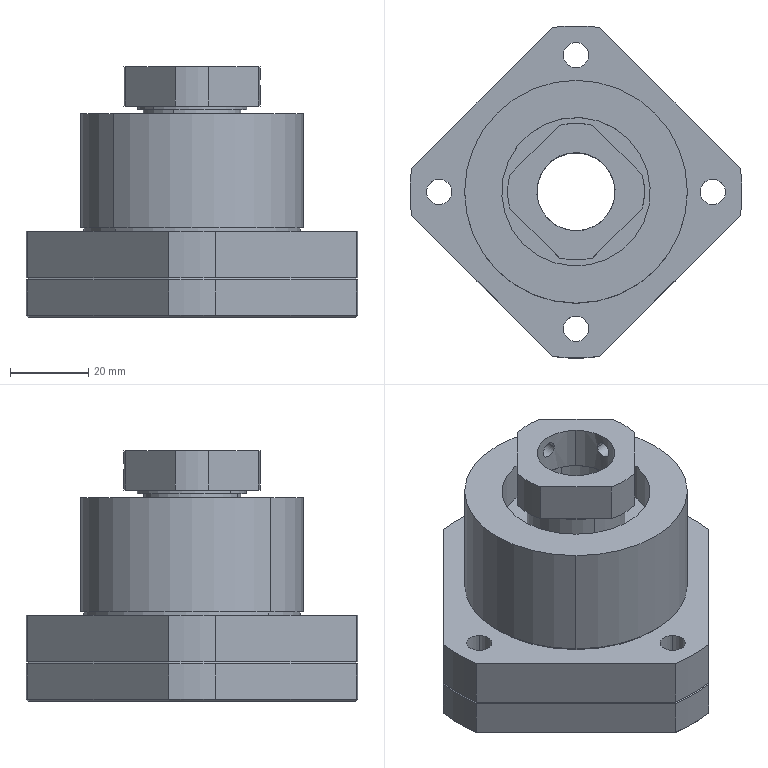Part | STEP file | TBI bearing block FK20 | 7 solids | 150 faces | box 85 x 85 x 64 mm | volume 139023 mm3 | cylinder 90 | plane 48 | cone 8 | spline 4 | commonest cylinder face diameters 6.5 x16 11 x16 20 x10 6 x8 47 x8 85 x8